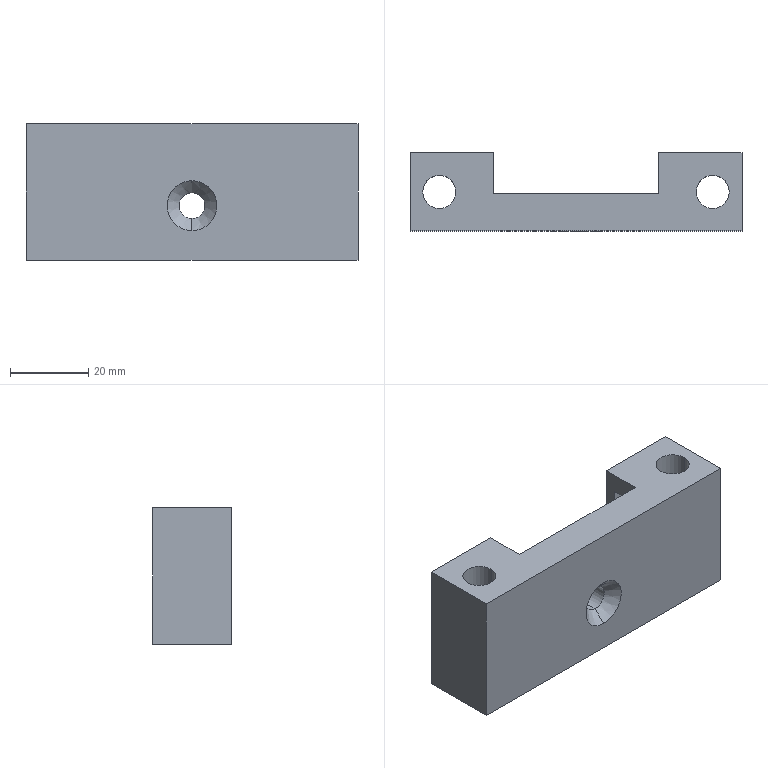Part | SolidWorks | features BaseBody 1, HoleWzd 1, MoveFace 1 | 1 solid | 30 faces | box 85 x 20 x 35 mm | volume 38495 mm3 | plane 18 | cylinder 10 | cone 2 | commonest cylinder face diameters 3 x4 8.5 x4 6.6 x2
STEP:
#1=CARTESIAN_POINT('',(0.,-6.9,17.3));
#2=VERTEX_POINT('',#1);
#3=CARTESIAN_POINT('',(0.,-6.9,10.7));
#4=VERTEX_POINT('',#3);
#5=CARTESIAN_POINT('',(0.,-6.9,14.));
#6=DIRECTION('',(0.,-1.,0.));
#7=DIRECTION('',(0.,0.,-1.));
#8=AXIS2_PLACEMENT_3D('',#5,#6,#7);
#9=CIRCLE('',#8,3.3);
#10=EDGE_CURVE('',#2,#4,#9,.T.);
#11=ORIENTED_EDGE('',*,*,#10,.F.);
#12=CARTESIAN_POINT('',(0.,-10.,20.4));
#13=VERTEX_POINT('',#12);
#14=CARTESIAN_POINT('',(0.,-10.,20.4));
#15=DIRECTION('',(0.,-0.7071,0.7071));
#16=VECTOR('',#15,1000.);
#17=LINE('',#14,#16);
#18=EDGE_CURVE('',#2,#13,#17,.T.);
#19=ORIENTED_EDGE('',*,*,#18,.T.);
#20=CARTESIAN_POINT('',(0.,-10.,7.6));
#21=VERTEX_POINT('',#20);
#22=CARTESIAN_POINT('',(0.,-10.,14.));
#23=DIRECTION('',(0.,-1.,0.));
#24=DIRECTION('',(0.,0.,-1.));
#25=AXIS2_PLACEMENT_3D('',#22,#23,#24);
#26=CIRCLE('',#25,6.4);
#27=EDGE_CURVE('',#13,#21,#26,.T.);
#28=ORIENTED_EDGE('',*,*,#27,.T.);
#29=CARTESIAN_POINT('',(0.,-10.,7.6));
#30=DIRECTION('',(0.,-0.7071,-0.7071));
#31=VECTOR('',#30,1000.);
#32=LINE('',#29,#31);
#33=EDGE_CURVE('',#4,#21,#32,.T.);
#34=ORIENTED_EDGE('',*,*,#33,.F.);
#35=EDGE_LOOP('',(#11,#19,#28,#34));
#36=FACE_OUTER_BOUND('',#35,.T.);
#37=CARTESIAN_POINT('',(0.,-10.,14.));
#38=DIRECTION('',(0.,-1.,0.));
#39=DIRECTION('',(0.,0.,-1.));
#40=AXIS2_PLACEMENT_3D('',#37,#38,#39);
#41=CONICAL_SURFACE('',#40,6.4,0.7854);
#42=ADVANCED_FACE('',(#36),#41,.F.);
#43=CARTESIAN_POINT('',(0.,-0.5,17.3));
#44=VERTEX_POINT('',#43);
#45=CARTESIAN_POINT('',(0.,-0.5,10.7));
#46=VERTEX_POINT('',#45);
#47=CARTESIAN_POINT('',(0.,-0.5,14.));
#48=DIRECTION('',(0.,-1.,0.));
#49=DIRECTION('',(1.,0.,0.));
#50=AXIS2_PLACEMENT_3D('',#47,#48,#49);
#51=CIRCLE('',#50,3.3);
#52=EDGE_CURVE('',#44,#46,#51,.T.);
#53=ORIENTED_EDGE('',*,*,#52,.F.);
#54=CARTESIAN_POINT('',(0.,-10.,17.3));
#55=DIRECTION('',(0.,-1.,0.));
#56=VECTOR('',#55,1000.);
#57=LINE('',#54,#56);
#58=EDGE_CURVE('',#44,#2,#57,.T.);
#59=ORIENTED_EDGE('',*,*,#58,.T.);
#60=ORIENTED_EDGE('',*,*,#10,.T.);
#61=CARTESIAN_POINT('',(0.,-10.,10.7));
#62=DIRECTION('',(0.,-1.,0.));
#63=VECTOR('',#62,1000.);
#64=LINE('',#61,#63);
#65=EDGE_CURVE('',#46,#4,#64,.T.);
#66=ORIENTED_EDGE('',*,*,#65,.F.);
#67=EDGE_LOOP('',(#53,#59,#60,#66));
#68=FACE_OUTER_BOUND('',#67,.T.);
#69=CARTESIAN_POINT('',(0.,-10.,14.));
#70=DIRECTION('',(0.,-1.,0.));
#71=DIRECTION('',(0.,0.,-1.));
#72=AXIS2_PLACEMENT_3D('',#69,#70,#71);
#73=CYLINDRICAL_SURFACE('',#72,3.3);
#74=ADVANCED_FACE('',(#68),#73,.F.);
#75=CARTESIAN_POINT('',(-39.25,0.,35.));
#76=VERTEX_POINT('',#75);
#77=CARTESIAN_POINT('',(-30.75,0.,35.));
#78=VERTEX_POINT('',#77);
#79=CARTESIAN_POINT('',(-35.,0.,35.));
#80=DIRECTION('',(0.,0.,1.));
#81=DIRECTION('',(1.,0.,0.));
#82=AXIS2_PLACEMENT_3D('',#79,#80,#81);
#83=CIRCLE('',#82,4.25);
#84=EDGE_CURVE('',#76,#78,#83,.T.);
#85=ORIENTED_EDGE('',*,*,#84,.T.);
#86=CARTESIAN_POINT('',(-30.75,0.,0.));
#87=VERTEX_POINT('',#86);
#88=CARTESIAN_POINT('',(-30.75,0.,0.));
#89=DIRECTION('',(0.,0.,-1.));
#90=VECTOR('',#89,1000.);
#91=LINE('',#88,#90);
#92=EDGE_CURVE('',#78,#87,#91,.T.);
#93=ORIENTED_EDGE('',*,*,#92,.T.);
#94=CARTESIAN_POINT('',(-39.25,0.,0.));
#95=VERTEX_POINT('',#94);
#96=CARTESIAN_POINT('',(-35.,0.,0.));
#97=DIRECTION('',(0.,0.,-1.));
#98=DIRECTION('',(-1.,0.,0.));
#99=AXIS2_PLACEMENT_3D('',#96,#97,#98);
#100=CIRCLE('',#99,4.25);
#101=EDGE_CURVE('',#87,#95,#100,.T.);
#102=ORIENTED_EDGE('',*,*,#101,.T.);
#103=CARTESIAN_POINT('',(-39.25,0.,0.));
#104=DIRECTION('',(0.,0.,-1.));
#105=VECTOR('',#104,1000.);
#106=LINE('',#103,#105);
#107=EDGE_CURVE('',#76,#95,#106,.T.);
#108=ORIENTED_EDGE('',*,*,#107,.F.);
#109=EDGE_LOOP('',(#85,#93,#102,#108));
#110=FACE_OUTER_BOUND('',#109,.T.);
#111=CARTESIAN_POINT('',(-35.,0.,0.));
#112=DIRECTION('',(0.,0.,-1.));
#113=DIRECTION('',(-1.,0.,0.));
#114=AXIS2_PLACEMENT_3D('',#111,#112,#113);
#115=CYLINDRICAL_SURFACE('',#114,4.25);
#116=ADVANCED_FACE('',(#110),#115,.F.);
#117=CARTESIAN_POINT('',(30.75,0.,35.));
#118=VERTEX_POINT('',#117);
#119=CARTESIAN_POINT('',(39.25,0.,35.));
#120=VERTEX_POINT('',#119);
#121=CARTESIAN_POINT('',(35.,0.,35.));
#122=DIRECTION('',(0.,0.,1.));
#123=DIRECTION('',(1.,0.,0.));
#124=AXIS2_PLACEMENT_3D('',#121,#122,#123);
#125=CIRCLE('',#124,4.25);
#126=EDGE_CURVE('',#118,#120,#125,.T.);
#127=ORIENTED_EDGE('',*,*,#126,.T.);
#128=CARTESIAN_POINT('',(39.25,0.,0.));
#129=VERTEX_POINT('',#128);
#130=CARTESIAN_POINT('',(39.25,0.,0.));
#131=DIRECTION('',(0.,0.,-1.));
#132=VECTOR('',#131,1000.);
#133=LINE('',#130,#132);
#134=EDGE_CURVE('',#120,#129,#133,.T.);
#135=ORIENTED_EDGE('',*,*,#134,.T.);
#136=CARTESIAN_POINT('',(30.75,0.,0.));
#137=VERTEX_POINT('',#136);
#138=CARTESIAN_POINT('',(35.,0.,0.));
#139=DIRECTION('',(0.,0.,-1.));
#140=DIRECTION('',(-1.,0.,0.));
#141=AXIS2_PLACEMENT_3D('',#138,#139,#140);
#142=CIRCLE('',#141,4.25);
#143=EDGE_CURVE('',#129,#137,#142,.T.);
#144=ORIENTED_EDGE('',*,*,#143,.T.);
#145=CARTESIAN_POINT('',(30.75,0.,0.));
#146=DIRECTION('',(0.,0.,-1.));
#147=VECTOR('',#146,1000.);
#148=LINE('',#145,#147);
#149=EDGE_CURVE('',#118,#137,#148,.T.);
#150=ORIENTED_EDGE('',*,*,#149,.F.);
#151=EDGE_LOOP('',(#127,#135,#144,#150));
#152=FACE_OUTER_BOUND('',#151,.T.);
#153=CARTESIAN_POINT('',(35.,0.,0.));
#154=DIRECTION('',(0.,0.,-1.));
#155=DIRECTION('',(-1.,0.,0.));
#156=AXIS2_PLACEMENT_3D('',#153,#154,#155);
#157=CYLINDRICAL_SURFACE('',#156,4.25);
#158=ADVANCED_FACE('',(#152),#157,.F.);
#159=CARTESIAN_POINT('',(23.5,7.,30.));
#160=VERTEX_POINT('',#159);
#161=CARTESIAN_POINT('',(25.,5.5,30.));
#162=VERTEX_POINT('',#161);
#163=CARTESIAN_POINT('',(23.5,5.5,30.));
#164=DIRECTION('',(0.,0.,-1.));
#165=DIRECTION('',(-1.,0.,0.));
#166=AXIS2_PLACEMENT_3D('',#163,#164,#165);
#167=CIRCLE('',#166,1.5);
#168=EDGE_CURVE('',#160,#162,#167,.T.);
#169=ORIENTED_EDGE('',*,*,#168,.F.);
#170=CARTESIAN_POINT('',(23.5,7.,0.));
#171=VERTEX_POINT('',#170);
#172=CARTESIAN_POINT('',(23.5,7.,30.));
#173=DIRECTION('',(0.,0.,1.));
#174=VECTOR('',#173,1000.);
#175=LINE('',#172,#174);
#176=EDGE_CURVE('',#171,#160,#175,.T.);
#177=ORIENTED_EDGE('',*,*,#176,.F.);
#178=CARTESIAN_POINT('',(25.,5.5,0.));
#179=VERTEX_POINT('',#178);
#180=CARTESIAN_POINT('',(23.5,5.5,0.));
#181=DIRECTION('',(0.,0.,1.));
#182=DIRECTION('',(1.,0.,0.));
#183=AXIS2_PLACEMENT_3D('',#180,#181,#182);
#184=CIRCLE('',#183,1.5);
#185=EDGE_CURVE('',#179,#171,#184,.T.);
#186=ORIENTED_EDGE('',*,*,#185,.F.);
#187=CARTESIAN_POINT('',(25.,5.5,0.));
#188=DIRECTION('',(0.,0.,-1.));
#189=VECTOR('',#188,1000.);
#190=LINE('',#187,#189);
#191=EDGE_CURVE('',#162,#179,#190,.T.);
#192=ORIENTED_EDGE('',*,*,#191,.F.);
#193=EDGE_LOOP('',(#169,#177,#186,#192));
#194=FACE_OUTER_BOUND('',#193,.T.);
#195=CARTESIAN_POINT('',(23.5,5.5,30.));
#196=DIRECTION('',(0.,0.,1.));
#197=DIRECTION('',(1.,0.,0.));
#198=AXIS2_PLACEMENT_3D('',#195,#196,#197);
#199=CYLINDRICAL_SURFACE('',#198,1.5);
#200=ADVANCED_FACE('',(#194),#199,.F.);
#201=CARTESIAN_POINT('',(25.,3.5,30.));
#202=VERTEX_POINT('',#201);
#203=CARTESIAN_POINT('',(23.5,2.,30.));
#204=VERTEX_POINT('',#203);
#205=CARTESIAN_POINT('',(23.5,3.5,30.));
#206=DIRECTION('',(0.,0.,-1.));
#207=DIRECTION('',(-1.,0.,0.));
#208=AXIS2_PLACEMENT_3D('',#205,#206,#207);
#209=CIRCLE('',#208,1.5);
#210=EDGE_CURVE('',#202,#204,#209,.T.);
#211=ORIENTED_EDGE('',*,*,#210,.F.);
#212=CARTESIAN_POINT('',(25.,3.5,0.));
#213=VERTEX_POINT('',#212);
#214=CARTESIAN_POINT('',(25.,3.5,30.));
#215=DIRECTION('',(0.,0.,1.));
#216=VECTOR('',#215,1000.);
#217=LINE('',#214,#216);
#218=EDGE_CURVE('',#213,#202,#217,.T.);
#219=ORIENTED_EDGE('',*,*,#218,.F.);
#220=CARTESIAN_POINT('',(23.5,2.,0.));
#221=VERTEX_POINT('',#220);
#222=CARTESIAN_POINT('',(23.5,3.5,0.));
#223=DIRECTION('',(0.,0.,1.));
#224=DIRECTION('',(1.,0.,0.));
#225=AXIS2_PLACEMENT_3D('',#222,#223,#224);
#226=CIRCLE('',#225,1.5);
#227=EDGE_CURVE('',#221,#213,#226,.T.);
#228=ORIENTED_EDGE('',*,*,#227,.F.);
#229=CARTESIAN_POINT('',(23.5,2.,0.));
#230=DIRECTION('',(0.,0.,-1.));
#231=VECTOR('',#230,1000.);
#232=LINE('',#229,#231);
#233=EDGE_CURVE('',#204,#221,#232,.T.);
#234=ORIENTED_EDGE('',*,*,#233,.F.);
#235=EDGE_LOOP('',(#211,#219,#228,#234));
#236=FACE_OUTER_BOUND('',#235,.T.);
#237=CARTESIAN_POINT('',(23.5,3.5,30.));
#238=DIRECTION('',(0.,0.,1.));
#239=DIRECTION('',(1.,0.,0.));
#240=AXIS2_PLACEMENT_3D('',#237,#238,#239);
#241=CYLINDRICAL_SURFACE('',#240,1.5);
#242=ADVANCED_FACE('',(#236),#241,.F.);
#243=CARTESIAN_POINT('',(-25.,5.5,30.));
#244=VERTEX_POINT('',#243);
#245=CARTESIAN_POINT('',(-23.5,7.,30.));
#246=VERTEX_POINT('',#245);
#247=CARTESIAN_POINT('',(-23.5,5.5,30.));
#248=DIRECTION('',(0.,0.,-1.));
#249=DIRECTION('',(-1.,0.,0.));
#250=AXIS2_PLACEMENT_3D('',#247,#248,#249);
#251=CIRCLE('',#250,1.5);
#252=EDGE_CURVE('',#244,#246,#251,.T.);
#253=ORIENTED_EDGE('',*,*,#252,.F.);
#254=CARTESIAN_POINT('',(-25.,5.5,0.));
#255=VERTEX_POINT('',#254);
#256=CARTESIAN_POINT('',(-25.,5.5,30.));
#257=DIRECTION('',(0.,0.,1.));
#258=VECTOR('',#257,1000.);
#259=LINE('',#256,#258);
#260=EDGE_CURVE('',#255,#244,#259,.T.);
#261=ORIENTED_EDGE('',*,*,#260,.F.);
#262=CARTESIAN_POINT('',(-23.5,7.,0.));
#263=VERTEX_POINT('',#262);
#264=CARTESIAN_POINT('',(-23.5,5.5,0.));
#265=DIRECTION('',(0.,0.,1.));
#266=DIRECTION('',(1.,0.,0.));
#267=AXIS2_PLACEMENT_3D('',#264,#265,#266);
#268=CIRCLE('',#267,1.5);
#269=EDGE_CURVE('',#263,#255,#268,.T.);
#270=ORIENTED_EDGE('',*,*,#269,.F.);
#271=CARTESIAN_POINT('',(-23.5,7.,0.));
#272=DIRECTION('',(0.,0.,-1.));
#273=VECTOR('',#272,1000.);
#274=LINE('',#271,#273);
#275=EDGE_CURVE('',#246,#263,#274,.T.);
#276=ORIENTED_EDGE('',*,*,#275,.F.);
#277=EDGE_LOOP('',(#253,#261,#270,#276));
#278=FACE_OUTER_BOUND('',#277,.T.);
#279=CARTESIAN_POINT('',(-23.5,5.5,30.));
#280=DIRECTION('',(0.,0.,1.));
#281=DIRECTION('',(1.,0.,0.));
#282=AXIS2_PLACEMENT_3D('',#279,#280,#281);
#283=CYLINDRICAL_SURFACE('',#282,1.5);
#284=ADVANCED_FACE('',(#278),#283,.F.);
#285=CARTESIAN_POINT('',(-23.5,2.,30.));
#286=VERTEX_POINT('',#285);
#287=CARTESIAN_POINT('',(-25.,3.5,30.));
#288=VERTEX_POINT('',#287);
#289=CARTESIAN_POINT('',(-23.5,3.5,30.));
#290=DIRECTION('',(0.,0.,-1.));
#291=DIRECTION('',(-1.,0.,0.));
#292=AXIS2_PLACEMENT_3D('',#289,#290,#291);
#293=CIRCLE('',#292,1.5);
#294=EDGE_CURVE('',#286,#288,#293,.T.);
#295=ORIENTED_EDGE('',*,*,#294,.F.);
#296=CARTESIAN_POINT('',(-23.5,2.,0.));
#297=VERTEX_POINT('',#296);
#298=CARTESIAN_POINT('',(-23.5,2.,30.));
#299=DIRECTION('',(0.,0.,1.));
#300=VECTOR('',#299,1000.);
#301=LINE('',#298,#300);
#302=EDGE_CURVE('',#297,#286,#301,.T.);
#303=ORIENTED_EDGE('',*,*,#302,.F.);
#304=CARTESIAN_POINT('',(-25.,3.5,0.));
#305=VERTEX_POINT('',#304);
#306=CARTESIAN_POINT('',(-23.5,3.5,0.));
#307=DIRECTION('',(0.,0.,1.));
#308=DIRECTION('',(1.,0.,0.));
#309=AXIS2_PLACEMENT_3D('',#306,#307,#308);
#310=CIRCLE('',#309,1.5);
#311=EDGE_CURVE('',#305,#297,#310,.T.);
#312=ORIENTED_EDGE('',*,*,#311,.F.);
#313=CARTESIAN_POINT('',(-25.,3.5,0.));
#314=DIRECTION('',(0.,0.,-1.));
#315=VECTOR('',#314,1000.);
#316=LINE('',#313,#315);
#317=EDGE_CURVE('',#288,#305,#316,.T.);
#318=ORIENTED_EDGE('',*,*,#317,.F.);
#319=EDGE_LOOP('',(#295,#303,#312,#318));
#320=FACE_OUTER_BOUND('',#319,.T.);
#321=CARTESIAN_POINT('',(-23.5,3.5,30.));
#322=DIRECTION('',(0.,0.,1.));
#323=DIRECTION('',(1.,0.,0.));
#324=AXIS2_PLACEMENT_3D('',#321,#322,#323);
#325=CYLINDRICAL_SURFACE('',#324,1.5);
#326=ADVANCED_FACE('',(#320),#325,.F.);
#327=CARTESIAN_POINT('',(-21.,2.,30.));
#328=VERTEX_POINT('',#327);
#329=CARTESIAN_POINT('',(-21.,2.,30.));
#330=DIRECTION('',(1.,0.,0.));
#331=VECTOR('',#330,1000.);
#332=LINE('',#329,#331);
#333=EDGE_CURVE('',#286,#328,#332,.T.);
#334=ORIENTED_EDGE('',*,*,#333,.F.);
#335=ORIENTED_EDGE('',*,*,#294,.T.);
#336=CARTESIAN_POINT('',(-25.,2.,30.));
#337=DIRECTION('',(0.,-1.,0.));
#338=VECTOR('',#337,1000.);
#339=LINE('',#336,#338);
#340=EDGE_CURVE('',#244,#288,#339,.T.);
#341=ORIENTED_EDGE('',*,*,#340,.F.);
#342=ORIENTED_EDGE('',*,*,#252,.T.);
#343=CARTESIAN_POINT('',(-21.,7.,30.));
#344=VERTEX_POINT('',#343);
#345=CARTESIAN_POINT('',(-21.,7.,30.));
#346=DIRECTION('',(-1.,0.,0.));
#347=VECTOR('',#346,1000.);
#348=LINE('',#345,#347);
#349=EDGE_CURVE('',#344,#246,#348,.T.);
#350=ORIENTED_EDGE('',*,*,#349,.F.);
#351=CARTESIAN_POINT('',(-21.,2.,30.));
#352=DIRECTION('',(0.,1.,0.));
#353=VECTOR('',#352,1000.);
#354=LINE('',#351,#353);
#355=EDGE_CURVE('',#328,#344,#354,.T.);
#356=ORIENTED_EDGE('',*,*,#355,.F.);
#357=EDGE_LOOP('',(#334,#335,#341,#342,#350,#356));
#358=FACE_OUTER_BOUND('',#357,.T.);
#359=CARTESIAN_POINT('',(0.,0.,30.));
#360=DIRECTION('',(0.,0.,-1.));
#361=DIRECTION('',(0.,-1.,0.));
#362=AXIS2_PLACEMENT_3D('',#359,#360,#361);
#363=PLANE('',#362);
#364=ADVANCED_FACE('',(#358),#363,.T.);
#365=CARTESIAN_POINT('',(-21.,2.,0.));
#366=VERTEX_POINT('',#365);
#367=CARTESIAN_POINT('',(-21.,2.,0.));
#368=DIRECTION('',(1.,0.,0.));
#369=VECTOR('',#368,1000.);
#370=LINE('',#367,#369);
#371=EDGE_CURVE('',#297,#366,#370,.T.);
#372=ORIENTED_EDGE('',*,*,#371,.F.);
#373=ORIENTED_EDGE('',*,*,#302,.T.);
#374=ORIENTED_EDGE('',*,*,#333,.T.);
#375=CARTESIAN_POINT('',(-21.,2.,30.));
#376=DIRECTION('',(0.,0.,-1.));
#377=VECTOR('',#376,1000.);
#378=LINE('',#375,#377);
#379=EDGE_CURVE('',#328,#366,#378,.T.);
#380=ORIENTED_EDGE('',*,*,#379,.T.);
#381=EDGE_LOOP('',(#372,#373,#374,#380));
#382=FACE_OUTER_BOUND('',#381,.T.);
#383=CARTESIAN_POINT('',(-21.,2.,30.));
#384=DIRECTION('',(0.,1.,0.));
#385=DIRECTION('',(1.,0.,0.));
#386=AXIS2_PLACEMENT_3D('',#383,#384,#385);
#387=PLANE('',#386);
#388=ADVANCED_FACE('',(#382),#387,.T.);
#389=ORIENTED_EDGE('',*,*,#340,.T.);
#390=ORIENTED_EDGE('',*,*,#317,.T.);
#391=CARTESIAN_POINT('',(-25.,2.,0.));
#392=DIRECTION('',(0.,-1.,0.));
#393=VECTOR('',#392,1000.);
#394=LINE('',#391,#393);
#395=EDGE_CURVE('',#255,#305,#394,.T.);
#396=ORIENTED_EDGE('',*,*,#395,.F.);
#397=ORIENTED_EDGE('',*,*,#260,.T.);
#398=EDGE_LOOP('',(#389,#390,#396,#397));
#399=FACE_OUTER_BOUND('',#398,.T.);
#400=CARTESIAN_POINT('',(-25.,2.,30.));
#401=DIRECTION('',(1.,0.,0.));
#402=DIRECTION('',(0.,1.,0.));
#403=AXIS2_PLACEMENT_3D('',#400,#401,#402);
#404=PLANE('',#403);
#405=ADVANCED_FACE('',(#399),#404,.T.);
#406=ORIENTED_EDGE('',*,*,#349,.T.);
#407=ORIENTED_EDGE('',*,*,#275,.T.);
#408=CARTESIAN_POINT('',(-21.,7.,0.));
#409=VERTEX_POINT('',#408);
#410=CARTESIAN_POINT('',(-21.,7.,0.));
#411=DIRECTION('',(-1.,0.,0.));
#412=VECTOR('',#411,1000.);
#413=LINE('',#410,#412);
#414=EDGE_CURVE('',#409,#263,#413,.T.);
#415=ORIENTED_EDGE('',*,*,#414,.F.);
#416=CARTESIAN_POINT('',(-21.,7.,30.));
#417=DIRECTION('',(0.,0.,-1.));
#418=VECTOR('',#417,1000.);
#419=LINE('',#416,#418);
#420=EDGE_CURVE('',#344,#409,#419,.T.);
#421=ORIENTED_EDGE('',*,*,#420,.F.);
#422=EDGE_LOOP('',(#406,#407,#415,#421));
#423=FACE_OUTER_BOUND('',#422,.T.);
#424=CARTESIAN_POINT('',(-21.,7.,30.));
#425=DIRECTION('',(0.,-1.,0.));
#426=DIRECTION('',(0.,0.,-1.));
#427=AXIS2_PLACEMENT_3D('',#424,#425,#426);
#428=PLANE('',#427);
#429=ADVANCED_FACE('',(#423),#428,.T.);
#430=CARTESIAN_POINT('',(25.,2.,30.));
#431=DIRECTION('',(0.,-1.,0.));
#432=VECTOR('',#431,1000.);
#433=LINE('',#430,#432);
#434=EDGE_CURVE('',#162,#202,#433,.T.);
#435=ORIENTED_EDGE('',*,*,#434,.T.);
#436=ORIENTED_EDGE('',*,*,#210,.T.);
#437=CARTESIAN_POINT('',(21.,2.,30.));
#438=VERTEX_POINT('',#437);
#439=CARTESIAN_POINT('',(21.,2.,30.));
#440=DIRECTION('',(-1.,0.,0.));
#441=VECTOR('',#440,1000.);
#442=LINE('',#439,#441);
#443=EDGE_CURVE('',#204,#438,#442,.T.);
#444=ORIENTED_EDGE('',*,*,#443,.T.);
#445=CARTESIAN_POINT('',(21.,7.,30.));
#446=VERTEX_POINT('',#445);
#447=CARTESIAN_POINT('',(21.,2.,30.));
#448=DIRECTION('',(0.,1.,0.));
#449=VECTOR('',#448,1000.);
#450=LINE('',#447,#449);
#451=EDGE_CURVE('',#438,#446,#450,.T.);
#452=ORIENTED_EDGE('',*,*,#451,.T.);
#453=CARTESIAN_POINT('',(21.,7.,30.));
#454=DIRECTION('',(1.,0.,0.));
#455=VECTOR('',#454,1000.);
#456=LINE('',#453,#455);
#457=EDGE_CURVE('',#446,#160,#456,.T.);
#458=ORIENTED_EDGE('',*,*,#457,.T.);
#459=ORIENTED_EDGE('',*,*,#168,.T.);
#460=EDGE_LOOP('',(#435,#436,#444,#452,#458,#459));
#461=FACE_OUTER_BOUND('',#460,.T.);
#462=CARTESIAN_POINT('',(0.,0.,30.));
#463=DIRECTION('',(0.,0.,-1.));
#464=DIRECTION('',(0.,-1.,0.));
#465=AXIS2_PLACEMENT_3D('',#462,#463,#464);
#466=PLANE('',#465);
#467=ADVANCED_FACE('',(#461),#466,.T.);
#468=CARTESIAN_POINT('',(21.,7.,0.));
#469=VERTEX_POINT('',#468);
#470=CARTESIAN_POINT('',(21.,7.,0.));
#471=DIRECTION('',(1.,0.,0.));
#472=VECTOR('',#471,1000.);
#473=LINE('',#470,#472);
#474=EDGE_CURVE('',#469,#171,#473,.T.);
#475=ORIENTED_EDGE('',*,*,#474,.T.);
#476=ORIENTED_EDGE('',*,*,#176,.T.);
#477=ORIENTED_EDGE('',*,*,#457,.F.);
#478=CARTESIAN_POINT('',(21.,7.,30.));
#479=DIRECTION('',(0.,0.,-1.));
#480=VECTOR('',#479,1000.);
#481=LINE('',#478,#480);
#482=EDGE_CURVE('',#446,#469,#481,.T.);
#483=ORIENTED_EDGE('',*,*,#482,.T.);
#484=EDGE_LOOP('',(#475,#476,#477,#483));
#485=FACE_OUTER_BOUND('',#484,.T.);
#486=CARTESIAN_POINT('',(21.,7.,30.));
#487=DIRECTION('',(0.,1.,0.));
#488=DIRECTION('',(1.,0.,0.));
#489=AXIS2_PLACEMENT_3D('',#486,#487,#488);
#490=PLANE('',#489);
#491=ADVANCED_FACE('',(#485),#490,.F.);
#492=CARTESIAN_POINT('',(25.,2.,0.));
#493=DIRECTION('',(0.,-1.,0.));
#494=VECTOR('',#493,1000.);
#495=LINE('',#492,#494);
#496=EDGE_CURVE('',#179,#213,#495,.T.);
#497=ORIENTED_EDGE('',*,*,#496,.T.);
#498=ORIENTED_EDGE('',*,*,#218,.T.);
#499=ORIENTED_EDGE('',*,*,#434,.F.);
#500=ORIENTED_EDGE('',*,*,#191,.T.);
#501=EDGE_LOOP('',(#497,#498,#499,#500));
#502=FACE_OUTER_BOUND('',#501,.T.);
#503=CARTESIAN_POINT('',(25.,2.,30.));
#504=DIRECTION('',(1.,0.,0.));
#505=DIRECTION('',(0.,1.,0.));
#506=AXIS2_PLACEMENT_3D('',#503,#504,#505);
#507=PLANE('',#506);
#508=ADVANCED_FACE('',(#502),#507,.F.);
#509=ORIENTED_EDGE('',*,*,#443,.F.);
#510=ORIENTED_EDGE('',*,*,#233,.T.);
#511=CARTESIAN_POINT('',(21.,2.,0.));
#512=VERTEX_POINT('',#511);
#513=CARTESIAN_POINT('',(21.,2.,0.));
#514=DIRECTION('',(-1.,0.,0.));
#515=VECTOR('',#514,1000.);
#516=LINE('',#513,#515);
#517=EDGE_CURVE('',#221,#512,#516,.T.);
#518=ORIENTED_EDGE('',*,*,#517,.T.);
#519=CARTESIAN_POINT('',(21.,2.,30.));
#520=DIRECTION('',(0.,0.,-1.));
#521=VECTOR('',#520,1000.);
#522=LINE('',#519,#521);
#523=EDGE_CURVE('',#438,#512,#522,.T.);
#524=ORIENTED_EDGE('',*,*,#523,.F.);
#525=EDGE_LOOP('',(#509,#510,#518,#524));
#526=FACE_OUTER_BOUND('',#525,.T.);
#527=CARTESIAN_POINT('',(21.,2.,30.));
#528=DIRECTION('',(0.,-1.,0.));
#529=DIRECTION('',(-1.,0.,0.));
#530=AXIS2_PLACEMENT_3D('',#527,#528,#529);
#531=PLANE('',#530);
#532=ADVANCED_FACE('',(#526),#531,.F.);
#533=CARTESIAN_POINT('',(0.,-0.5,14.));
#534=DIRECTION('',(0.,-1.,0.));
#535=DIRECTION('',(1.,0.,0.));
#536=AXIS2_PLACEMENT_3D('',#533,#534,#535);
#537=CIRCLE('',#536,3.3);
#538=EDGE_CURVE('',#46,#44,#537,.T.);
#539=ORIENTED_EDGE('',*,*,#538,.T.);
#540=ORIENTED_EDGE('',*,*,#52,.T.);
#541=EDGE_LOOP('',(#539,#540));
#542=FACE_BOUND('',#541,.T.);
#543=CARTESIAN_POINT('',(-21.,-0.5,35.));
#544=VERTEX_POINT('',#543);
#545=CARTESIAN_POINT('',(21.,-0.5,35.));
#546=VERTEX_POINT('',#545);
#547=CARTESIAN_POINT('',(0.,-0.5,35.));
#548=DIRECTION('',(1.,0.,0.));
#549=VECTOR('',#548,1000.);
#550=LINE('',#547,#549);
#551=EDGE_CURVE('',#544,#546,#550,.T.);
#552=ORIENTED_EDGE('',*,*,#551,.T.);
#553=CARTESIAN_POINT('',(21.,-0.5,0.));
#554=VERTEX_POINT('',#553);
#555=CARTESIAN_POINT('',(21.,-0.5,50.));
#556=DIRECTION('',(0.,0.,-1.));
#557=VECTOR('',#556,1000.);
#558=LINE('',#555,#557);
#559=EDGE_CURVE('',#546,#554,#558,.T.);
#560=ORIENTED_EDGE('',*,*,#559,.T.);
#561=CARTESIAN_POINT('',(-21.,-0.5,0.));
#562=VERTEX_POINT('',#561);
#563=CARTESIAN_POINT('',(21.,-0.5,0.));
#564=DIRECTION('',(-1.,0.,0.));
#565=VECTOR('',#564,1000.);
#566=LINE('',#563,#565);
#567=EDGE_CURVE('',#554,#562,#566,.T.);
#568=ORIENTED_EDGE('',*,*,#567,.T.);
#569=CARTESIAN_POINT('',(-21.,-0.5,50.));
#570=DIRECTION('',(0.,0.,-1.));
#571=VECTOR('',#570,1000.);
#572=LINE('',#569,#571);
#573=EDGE_CURVE('',#544,#562,#572,.T.);
#574=ORIENTED_EDGE('',*,*,#573,.F.);
#575=EDGE_LOOP('',(#552,#560,#568,#574));
#576=FACE_OUTER_BOUND('',#575,.T.);
#577=CARTESIAN_POINT('',(21.,-0.5,50.));
#578=DIRECTION('',(0.,-1.,0.));
#579=DIRECTION('',(-1.,0.,0.));
#580=AXIS2_PLACEMENT_3D('',#577,#578,#579);
#581=PLANE('',#580);
#582=ADVANCED_FACE('',(#542,#576),#581,.F.);
#583=ORIENTED_EDGE('',*,*,#451,.F.);
#584=ORIENTED_EDGE('',*,*,#523,.T.);
#585=CARTESIAN_POINT('',(21.,10.,0.));
#586=DIRECTION('',(0.,-1.,0.));
#587=VECTOR('',#586,1000.);
#588=LINE('',#585,#587);
#589=EDGE_CURVE('',#512,#554,#588,.T.);
#590=ORIENTED_EDGE('',*,*,#589,.T.);
#591=ORIENTED_EDGE('',*,*,#559,.F.);
#592=CARTESIAN_POINT('',(21.,10.,35.));
#593=VERTEX_POINT('',#592);
#594=CARTESIAN_POINT('',(21.,0.,35.));
#595=DIRECTION('',(0.,1.,0.));
#596=VECTOR('',#595,1000.);
#597=LINE('',#594,#596);
#598=EDGE_CURVE('',#546,#593,#597,.T.);
#599=ORIENTED_EDGE('',*,*,#598,.T.);
#600=CARTESIAN_POINT('',(21.,10.,0.));
#601=VERTEX_POINT('',#600);
#602=CARTESIAN_POINT('',(21.,10.,50.));
#603=DIRECTION('',(0.,0.,-1.));
#604=VECTOR('',#603,1000.);
#605=LINE('',#602,#604);
#606=EDGE_CURVE('',#593,#601,#605,.T.);
#607=ORIENTED_EDGE('',*,*,#606,.T.);
#608=CARTESIAN_POINT('',(21.,10.,0.));
#609=DIRECTION('',(0.,-1.,0.));
#610=VECTOR('',#609,1000.);
#611=LINE('',#608,#610);
#612=EDGE_CURVE('',#601,#469,#611,.T.);
#613=ORIENTED_EDGE('',*,*,#612,.T.);
#614=ORIENTED_EDGE('',*,*,#482,.F.);
#615=EDGE_LOOP('',(#583,#584,#590,#591,#599,#607,#613,#614));
#616=FACE_OUTER_BOUND('',#615,.T.);
#617=CARTESIAN_POINT('',(21.,10.,50.));
#618=DIRECTION('',(1.,0.,0.));
#619=DIRECTION('',(0.,-1.,0.));
#620=AXIS2_PLACEMENT_3D('',#617,#618,#619);
#621=PLANE('',#620);
#622=ADVANCED_FACE('',(#616),#621,.F.);
#623=ORIENTED_EDGE('',*,*,#126,.F.);
#624=CARTESIAN_POINT('',(35.,0.,35.));
#625=DIRECTION('',(0.,0.,1.));
#626=DIRECTION('',(1.,0.,0.));
#627=AXIS2_PLACEMENT_3D('',#624,#625,#626);
#628=CIRCLE('',#627,4.25);
#629=EDGE_CURVE('',#120,#118,#628,.T.);
#630=ORIENTED_EDGE('',*,*,#629,.F.);
#631=EDGE_LOOP('',(#623,#630));
#632=FACE_BOUND('',#631,.T.);
#633=ORIENTED_EDGE('',*,*,#84,.F.);
#634=CARTESIAN_POINT('',(-35.,0.,35.));
#635=DIRECTION('',(0.,0.,1.));
#636=DIRECTION('',(1.,0.,0.));
#637=AXIS2_PLACEMENT_3D('',#634,#635,#636);
#638=CIRCLE('',#637,4.25);
#639=EDGE_CURVE('',#78,#76,#638,.T.);
#640=ORIENTED_EDGE('',*,*,#639,.F.);
#641=EDGE_LOOP('',(#633,#640));
#642=FACE_BOUND('',#641,.T.);
#643=ORIENTED_EDGE('',*,*,#598,.F.);
#644=ORIENTED_EDGE('',*,*,#551,.F.);
#645=CARTESIAN_POINT('',(-21.,10.,35.));
#646=VERTEX_POINT('',#645);
#647=CARTESIAN_POINT('',(-21.,0.,35.));
#648=DIRECTION('',(0.,-1.,0.));
#649=VECTOR('',#648,1000.);
#650=LINE('',#647,#649);
#651=EDGE_CURVE('',#646,#544,#650,.T.);
#652=ORIENTED_EDGE('',*,*,#651,.F.);
#653=CARTESIAN_POINT('',(-42.5,10.,35.));
#654=VERTEX_POINT('',#653);
#655=CARTESIAN_POINT('',(-42.5,10.,35.));
#656=DIRECTION('',(-1.,0.,0.));
#657=VECTOR('',#656,1000.);
#658=LINE('',#655,#657);
#659=EDGE_CURVE('',#646,#654,#658,.T.);
#660=ORIENTED_EDGE('',*,*,#659,.T.);
#661=CARTESIAN_POINT('',(-42.5,-10.,35.));
#662=VERTEX_POINT('',#661);
#663=CARTESIAN_POINT('',(-42.5,10.,35.));
#664=DIRECTION('',(0.,-1.,0.));
#665=VECTOR('',#664,1000.);
#666=LINE('',#663,#665);
#667=EDGE_CURVE('',#654,#662,#666,.T.);
#668=ORIENTED_EDGE('',*,*,#667,.T.);
#669=CARTESIAN_POINT('',(42.5,-10.,35.));
#670=VERTEX_POINT('',#669);
#671=CARTESIAN_POINT('',(-42.5,-10.,35.));
#672=DIRECTION('',(1.,0.,0.));
#673=VECTOR('',#672,1000.);
#674=LINE('',#671,#673);
#675=EDGE_CURVE('',#662,#670,#674,.T.);
#676=ORIENTED_EDGE('',*,*,#675,.T.);
#677=CARTESIAN_POINT('',(42.5,10.,35.));
#678=VERTEX_POINT('',#677);
#679=CARTESIAN_POINT('',(42.5,10.,35.));
#680=DIRECTION('',(0.,1.,0.));
#681=VECTOR('',#680,1000.);
#682=LINE('',#679,#681);
#683=EDGE_CURVE('',#670,#678,#682,.T.);
#684=ORIENTED_EDGE('',*,*,#683,.T.);
#685=CARTESIAN_POINT('',(-42.5,10.,35.));
#686=DIRECTION('',(-1.,0.,0.));
#687=VECTOR('',#686,1000.);
#688=LINE('',#685,#687);
#689=EDGE_CURVE('',#678,#593,#688,.T.);
#690=ORIENTED_EDGE('',*,*,#689,.T.);
#691=EDGE_LOOP('',(#643,#644,#652,#660,#668,#676,#684,#690));
#692=FACE_OUTER_BOUND('',#691,.T.);
#693=CARTESIAN_POINT('',(0.,0.,35.));
#694=DIRECTION('',(0.,0.,1.));
#695=DIRECTION('',(1.,0.,0.));
#696=AXIS2_PLACEMENT_3D('',#693,#694,#695);
#697=PLANE('',#696);
#698=ADVANCED_FACE('',(#632,#642,#692),#697,.T.);
#699=CARTESIAN_POINT('',(0.,-10.,14.));
#700=DIRECTION('',(0.,-1.,0.));
#701=DIRECTION('',(0.,0.,-1.));
#702=AXIS2_PLACEMENT_3D('',#699,#700,#701);
#703=CIRCLE('',#702,6.4);
#704=EDGE_CURVE('',#21,#13,#703,.T.);
#705=ORIENTED_EDGE('',*,*,#704,.F.);
#706=ORIENTED_EDGE('',*,*,#27,.F.);
#707=EDGE_LOOP('',(#705,#706));
#708=FACE_BOUND('',#707,.T.);
#709=CARTESIAN_POINT('',(-42.5,-10.,0.));
#710=VERTEX_POINT('',#709);
#711=CARTESIAN_POINT('',(42.5,-10.,0.));
#712=VERTEX_POINT('',#711);
#713=CARTESIAN_POINT('',(-42.5,-10.,0.));
#714=DIRECTION('',(1.,0.,0.));
#715=VECTOR('',#714,1000.);
#716=LINE('',#713,#715);
#717=EDGE_CURVE('',#710,#712,#716,.T.);
#718=ORIENTED_EDGE('',*,*,#717,.T.);
#719=CARTESIAN_POINT('',(42.5,-10.,35.));
#720=DIRECTION('',(0.,0.,-1.));
#721=VECTOR('',#720,1000.);
#722=LINE('',#719,#721);
#723=EDGE_CURVE('',#670,#712,#722,.T.);
#724=ORIENTED_EDGE('',*,*,#723,.F.);
#725=ORIENTED_EDGE('',*,*,#675,.F.);
#726=CARTESIAN_POINT('',(-42.5,-10.,35.));
#727=DIRECTION('',(0.,0.,-1.));
#728=VECTOR('',#727,1000.);
#729=LINE('',#726,#728);
#730=EDGE_CURVE('',#662,#710,#729,.T.);
#731=ORIENTED_EDGE('',*,*,#730,.T.);
#732=EDGE_LOOP('',(#718,#724,#725,#731));
#733=FACE_OUTER_BOUND('',#732,.T.);
#734=CARTESIAN_POINT('',(-42.5,-10.,35.));
#735=DIRECTION('',(0.,1.,0.));
#736=DIRECTION('',(1.,0.,0.));
#737=AXIS2_PLACEMENT_3D('',#734,#735,#736);
#738=PLANE('',#737);
#739=ADVANCED_FACE('',(#708,#733),#738,.F.);
#740=CARTESIAN_POINT('',(-42.5,10.,0.));
#741=VERTEX_POINT('',#740);
#742=CARTESIAN_POINT('',(-42.5,10.,0.));
#743=DIRECTION('',(0.,-1.,0.));
#744=VECTOR('',#743,1000.);
#745=LINE('',#742,#744);
#746=EDGE_CURVE('',#741,#710,#745,.T.);
#747=ORIENTED_EDGE('',*,*,#746,.T.);
#748=ORIENTED_EDGE('',*,*,#730,.F.);
#749=ORIENTED_EDGE('',*,*,#667,.F.);
#750=CARTESIAN_POINT('',(-42.5,10.,35.));
#751=DIRECTION('',(0.,0.,-1.));
#752=VECTOR('',#751,1000.);
#753=LINE('',#750,#752);
#754=EDGE_CURVE('',#654,#741,#753,.T.);
#755=ORIENTED_EDGE('',*,*,#754,.T.);
#756=EDGE_LOOP('',(#747,#748,#749,#755));
#757=FACE_OUTER_BOUND('',#756,.T.);
#758=CARTESIAN_POINT('',(-42.5,10.,35.));
#759=DIRECTION('',(1.,0.,0.));
#760=DIRECTION('',(0.,-1.,0.));
#761=AXIS2_PLACEMENT_3D('',#758,#759,#760);
#762=PLANE('',#761);
#763=ADVANCED_FACE('',(#757),#762,.F.);
#764=ORIENTED_EDGE('',*,*,#659,.F.);
#765=CARTESIAN_POINT('',(-21.,10.,0.));
#766=VERTEX_POINT('',#765);
#767=CARTESIAN_POINT('',(-21.,10.,50.));
#768=DIRECTION('',(0.,0.,-1.));
#769=VECTOR('',#768,1000.);
#770=LINE('',#767,#769);
#771=EDGE_CURVE('',#646,#766,#770,.T.);
#772=ORIENTED_EDGE('',*,*,#771,.T.);
#773=CARTESIAN_POINT('',(-42.5,10.,0.));
#774=DIRECTION('',(-1.,0.,0.));
#775=VECTOR('',#774,1000.);
#776=LINE('',#773,#775);
#777=EDGE_CURVE('',#766,#741,#776,.T.);
#778=ORIENTED_EDGE('',*,*,#777,.T.);
#779=ORIENTED_EDGE('',*,*,#754,.F.);
#780=EDGE_LOOP('',(#764,#772,#778,#779));
#781=FACE_OUTER_BOUND('',#780,.T.);
#782=CARTESIAN_POINT('',(-42.5,10.,35.));
#783=DIRECTION('',(0.,-1.,0.));
#784=DIRECTION('',(0.,0.,-1.));
#785=AXIS2_PLACEMENT_3D('',#782,#783,#784);
#786=PLANE('',#785);
#787=ADVANCED_FACE('',(#781),#786,.F.);
#788=CARTESIAN_POINT('',(42.5,10.,0.));
#789=VERTEX_POINT('',#788);
#790=CARTESIAN_POINT('',(42.5,10.,0.));
#791=DIRECTION('',(0.,1.,0.));
#792=VECTOR('',#791,1000.);
#793=LINE('',#790,#792);
#794=EDGE_CURVE('',#712,#789,#793,.T.);
#795=ORIENTED_EDGE('',*,*,#794,.T.);
#796=CARTESIAN_POINT('',(42.5,10.,35.));
#797=DIRECTION('',(0.,0.,-1.));
#798=VECTOR('',#797,1000.);
#799=LINE('',#796,#798);
#800=EDGE_CURVE('',#678,#789,#799,.T.);
#801=ORIENTED_EDGE('',*,*,#800,.F.);
#802=ORIENTED_EDGE('',*,*,#683,.F.);
#803=ORIENTED_EDGE('',*,*,#723,.T.);
#804=EDGE_LOOP('',(#795,#801,#802,#803));
#805=FACE_OUTER_BOUND('',#804,.T.);
#806=CARTESIAN_POINT('',(42.5,10.,35.));
#807=DIRECTION('',(-1.,0.,0.));
#808=DIRECTION('',(0.,1.,0.));
#809=AXIS2_PLACEMENT_3D('',#806,#807,#808);
#810=PLANE('',#809);
#811=ADVANCED_FACE('',(#805),#810,.F.);
#812=CARTESIAN_POINT('',(-42.5,10.,0.));
#813=DIRECTION('',(-1.,0.,0.));
#814=VECTOR('',#813,1000.);
#815=LINE('',#812,#814);
#816=EDGE_CURVE('',#789,#601,#815,.T.);
#817=ORIENTED_EDGE('',*,*,#816,.T.);
#818=ORIENTED_EDGE('',*,*,#606,.F.);
#819=ORIENTED_EDGE('',*,*,#689,.F.);
#820=ORIENTED_EDGE('',*,*,#800,.T.);
#821=EDGE_LOOP('',(#817,#818,#819,#820));
#822=FACE_OUTER_BOUND('',#821,.T.);
#823=CARTESIAN_POINT('',(-42.5,10.,35.));
#824=DIRECTION('',(0.,-1.,0.));
#825=DIRECTION('',(0.,0.,-1.));
#826=AXIS2_PLACEMENT_3D('',#823,#824,#825);
#827=PLANE('',#826);
#828=ADVANCED_FACE('',(#822),#827,.F.);
#829=ORIENTED_EDGE('',*,*,#420,.T.);
#830=CARTESIAN_POINT('',(-21.,10.,0.));
#831=DIRECTION('',(0.,1.,0.));
#832=VECTOR('',#831,1000.);
#833=LINE('',#830,#832);
#834=EDGE_CURVE('',#409,#766,#833,.T.);
#835=ORIENTED_EDGE('',*,*,#834,.T.);
#836=ORIENTED_EDGE('',*,*,#771,.F.);
#837=ORIENTED_EDGE('',*,*,#651,.T.);
#838=ORIENTED_EDGE('',*,*,#573,.T.);
#839=CARTESIAN_POINT('',(-21.,10.,0.));
#840=DIRECTION('',(0.,1.,0.));
#841=VECTOR('',#840,1000.);
#842=LINE('',#839,#841);
#843=EDGE_CURVE('',#562,#366,#842,.T.);
#844=ORIENTED_EDGE('',*,*,#843,.T.);
#845=ORIENTED_EDGE('',*,*,#379,.F.);
#846=ORIENTED_EDGE('',*,*,#355,.T.);
#847=EDGE_LOOP('',(#829,#835,#836,#837,#838,#844,#845,#846));
#848=FACE_OUTER_BOUND('',#847,.T.);
#849=CARTESIAN_POINT('',(-21.,10.,50.));
#850=DIRECTION('',(-1.,0.,0.));
#851=DIRECTION('',(0.,1.,0.));
#852=AXIS2_PLACEMENT_3D('',#849,#850,#851);
#853=PLANE('',#852);
#854=ADVANCED_FACE('',(#848),#853,.F.);
#855=CARTESIAN_POINT('',(35.,0.,0.));
#856=DIRECTION('',(0.,0.,-1.));
#857=DIRECTION('',(-1.,0.,0.));
#858=AXIS2_PLACEMENT_3D('',#855,#856,#857);
#859=CIRCLE('',#858,4.25);
#860=EDGE_CURVE('',#137,#129,#859,.T.);
#861=ORIENTED_EDGE('',*,*,#860,.F.);
#862=ORIENTED_EDGE('',*,*,#143,.F.);
#863=EDGE_LOOP('',(#861,#862));
#864=FACE_BOUND('',#863,.T.);
#865=CARTESIAN_POINT('',(-35.,0.,0.));
#866=DIRECTION('',(0.,0.,-1.));
#867=DIRECTION('',(-1.,0.,0.));
#868=AXIS2_PLACEMENT_3D('',#865,#866,#867);
#869=CIRCLE('',#868,4.25);
#870=EDGE_CURVE('',#95,#87,#869,.T.);
#871=ORIENTED_EDGE('',*,*,#870,.F.);
#872=ORIENTED_EDGE('',*,*,#101,.F.);
#873=EDGE_LOOP('',(#871,#872));
#874=FACE_BOUND('',#873,.T.);
#875=ORIENTED_EDGE('',*,*,#414,.T.);
#876=ORIENTED_EDGE('',*,*,#269,.T.);
#877=ORIENTED_EDGE('',*,*,#395,.T.);
#878=ORIENTED_EDGE('',*,*,#311,.T.);
#879=ORIENTED_EDGE('',*,*,#371,.T.);
#880=ORIENTED_EDGE('',*,*,#843,.F.);
#881=ORIENTED_EDGE('',*,*,#567,.F.);
#882=ORIENTED_EDGE('',*,*,#589,.F.);
#883=ORIENTED_EDGE('',*,*,#517,.F.);
#884=ORIENTED_EDGE('',*,*,#227,.T.);
#885=ORIENTED_EDGE('',*,*,#496,.F.);
#886=ORIENTED_EDGE('',*,*,#185,.T.);
#887=ORIENTED_EDGE('',*,*,#474,.F.);
#888=ORIENTED_EDGE('',*,*,#612,.F.);
#889=ORIENTED_EDGE('',*,*,#816,.F.);
#890=ORIENTED_EDGE('',*,*,#794,.F.);
#891=ORIENTED_EDGE('',*,*,#717,.F.);
#892=ORIENTED_EDGE('',*,*,#746,.F.);
#893=ORIENTED_EDGE('',*,*,#777,.F.);
#894=ORIENTED_EDGE('',*,*,#834,.F.);
#895=EDGE_LOOP('',(#875,#876,#877,#878,#879,#880,#881,#882,#883,#884,#885,#886,#887,#888,#889,#890,#891,#892,#893,#894));
#896=FACE_OUTER_BOUND('',#895,.T.);
#897=CARTESIAN_POINT('',(0.,0.,0.));
#898=DIRECTION('',(0.,0.,1.));
#899=DIRECTION('',(1.,0.,0.));
#900=AXIS2_PLACEMENT_3D('',#897,#898,#899);
#901=PLANE('',#900);
#902=ADVANCED_FACE('',(#864,#874,#896),#901,.F.);
#903=ORIENTED_EDGE('',*,*,#134,.F.);
#904=ORIENTED_EDGE('',*,*,#629,.T.);
#905=ORIENTED_EDGE('',*,*,#149,.T.);
#906=ORIENTED_EDGE('',*,*,#860,.T.);
#907=EDGE_LOOP('',(#903,#904,#905,#906));
#908=FACE_OUTER_BOUND('',#907,.T.);
#909=CARTESIAN_POINT('',(35.,0.,0.));
#910=DIRECTION('',(0.,0.,-1.));
#911=DIRECTION('',(-1.,0.,0.));
#912=AXIS2_PLACEMENT_3D('',#909,#910,#911);
#913=CYLINDRICAL_SURFACE('',#912,4.25);
#914=ADVANCED_FACE('',(#908),#913,.F.);
#915=ORIENTED_EDGE('',*,*,#92,.F.);
#916=ORIENTED_EDGE('',*,*,#639,.T.);
#917=ORIENTED_EDGE('',*,*,#107,.T.);
#918=ORIENTED_EDGE('',*,*,#870,.T.);
#919=EDGE_LOOP('',(#915,#916,#917,#918));
#920=FACE_OUTER_BOUND('',#919,.T.);
#921=CARTESIAN_POINT('',(-35.,0.,0.));
#922=DIRECTION('',(0.,0.,-1.));
#923=DIRECTION('',(-1.,0.,0.));
#924=AXIS2_PLACEMENT_3D('',#921,#922,#923);
#925=CYLINDRICAL_SURFACE('',#924,4.25);
#926=ADVANCED_FACE('',(#920),#925,.F.);
#927=ORIENTED_EDGE('',*,*,#58,.F.);
#928=ORIENTED_EDGE('',*,*,#538,.F.);
#929=ORIENTED_EDGE('',*,*,#65,.T.);
#930=CARTESIAN_POINT('',(0.,-6.9,14.));
#931=DIRECTION('',(0.,-1.,0.));
#932=DIRECTION('',(0.,0.,-1.));
#933=AXIS2_PLACEMENT_3D('',#930,#931,#932);
#934=CIRCLE('',#933,3.3);
#935=EDGE_CURVE('',#4,#2,#934,.T.);
#936=ORIENTED_EDGE('',*,*,#935,.T.);
#937=EDGE_LOOP('',(#927,#928,#929,#936));
#938=FACE_OUTER_BOUND('',#937,.T.);
#939=CARTESIAN_POINT('',(0.,-10.,14.));
#940=DIRECTION('',(0.,-1.,0.));
#941=DIRECTION('',(0.,0.,-1.));
#942=AXIS2_PLACEMENT_3D('',#939,#940,#941);
#943=CYLINDRICAL_SURFACE('',#942,3.3);
#944=ADVANCED_FACE('',(#938),#943,.F.);
#945=ORIENTED_EDGE('',*,*,#18,.F.);
#946=ORIENTED_EDGE('',*,*,#935,.F.);
#947=ORIENTED_EDGE('',*,*,#33,.T.);
#948=ORIENTED_EDGE('',*,*,#704,.T.);
#949=EDGE_LOOP('',(#945,#946,#947,#948));
#950=FACE_OUTER_BOUND('',#949,.T.);
#951=CARTESIAN_POINT('',(0.,-10.,14.));
#952=DIRECTION('',(0.,-1.,0.));
#953=DIRECTION('',(0.,0.,-1.));
#954=AXIS2_PLACEMENT_3D('',#951,#952,#953);
#955=CONICAL_SURFACE('',#954,6.4,0.7854);
#956=ADVANCED_FACE('',(#950),#955,.F.);
#957=CLOSED_SHELL('',(#42,#74,#116,#158,#200,#242,#284,#326,#364,#388,#405,#429,#467,#491,#508,#532,#582,#622,#698,#739,#763,#787,#811,#828,#854,#902,#914,#926,#944,#956));
#958=MANIFOLD_SOLID_BREP('',#957);
#959=CARTESIAN_POINT('',(0.,0.,0.));
#960=DIRECTION('',(0.,0.,1.));
#961=DIRECTION('',(1.,0.,0.));
#962=AXIS2_PLACEMENT_3D('',#959,#960,#961);
#963=(LENGTH_UNIT()NAMED_UNIT(*)SI_UNIT(.MILLI.,.METRE.));
#964=UNCERTAINTY_MEASURE_WITH_UNIT(LENGTH_MEASURE(0.00001),#963,'','');
#965=(NAMED_UNIT(*)PLANE_ANGLE_UNIT()SI_UNIT($,.RADIAN.));
#966=(NAMED_UNIT(*)SI_UNIT($,.STERADIAN.)SOLID_ANGLE_UNIT());
#967=(GEOMETRIC_REPRESENTATION_CONTEXT(3)GLOBAL_UNCERTAINTY_ASSIGNED_CONTEXT((#964))GLOBAL_UNIT_ASSIGNED_CONTEXT((#963,#965,#966))REPRESENTATION_CONTEXT('',''));
#968=ADVANCED_BREP_SHAPE_REPRESENTATION('',(#958,#962),#967);